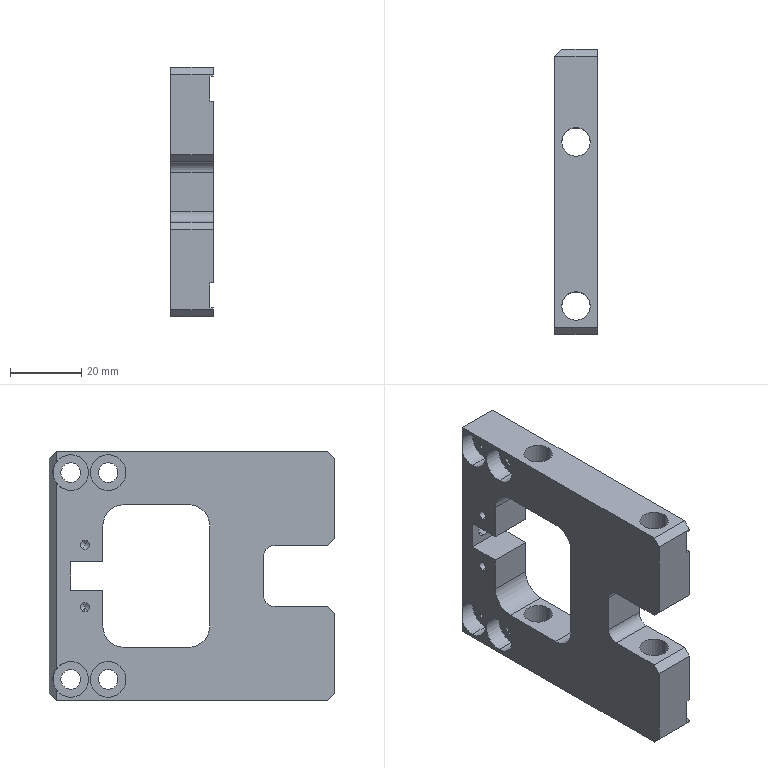Part | NX | features BREP 1 | 1 solid | 79 faces | box 12 x 80 x 70 mm | volume 40311 mm3 | plane 39 | cylinder 36 | cone 4 | commonest cylinder face diameters 5.5 x8 8 x8 10 x8 2.5 x4 12 x4 4.1 x2